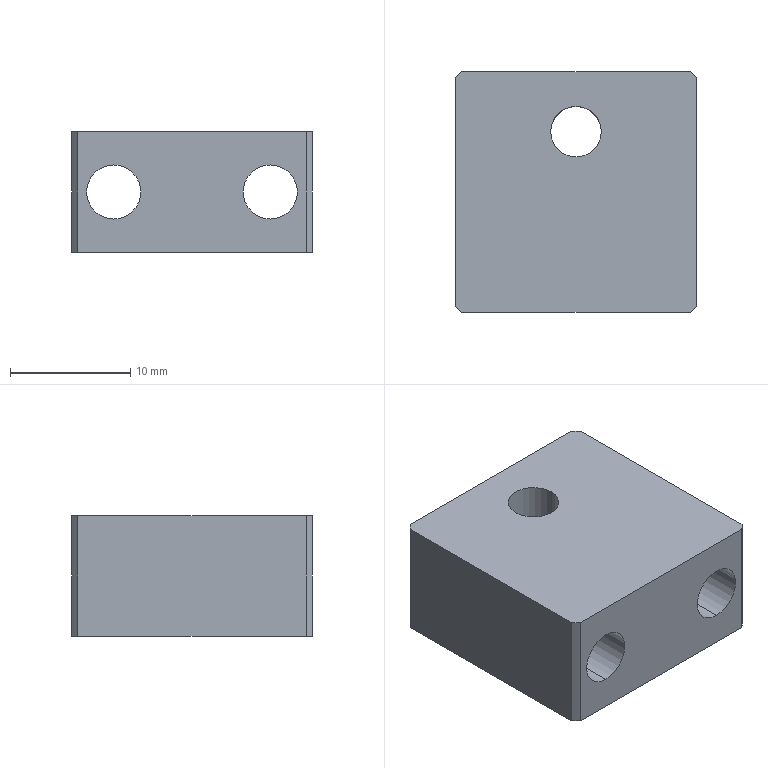Part | SolidWorks | features HoleWzd 2, Chamfer 1, Extrusion 1 | 1 solid | 16 faces | box 20 x 20 x 10 mm | volume 3220 mm3 | plane 10 | cylinder 6 | commonest cylinder face diameters 4.5 x4 4.2 x2
STEP:
#1=CARTESIAN_POINT('',(-6.5,-10.,-2.25));
#2=VERTEX_POINT('',#1);
#3=CARTESIAN_POINT('',(-6.5,-10.,2.25));
#4=VERTEX_POINT('',#3);
#5=CARTESIAN_POINT('',(-6.5,-10.,0.));
#6=DIRECTION('',(0.,1.,0.));
#7=DIRECTION('',(0.,0.,1.));
#8=AXIS2_PLACEMENT_3D('',#5,#6,#7);
#9=CIRCLE('',#8,2.25);
#10=EDGE_CURVE('',#2,#4,#9,.T.);
#11=ORIENTED_EDGE('',*,*,#10,.F.);
#12=CARTESIAN_POINT('',(-6.5,10.,-2.25));
#13=VERTEX_POINT('',#12);
#14=CARTESIAN_POINT('',(-6.5,10.,-2.25));
#15=DIRECTION('',(0.,1.,0.));
#16=VECTOR('',#15,1000.);
#17=LINE('',#14,#16);
#18=EDGE_CURVE('',#2,#13,#17,.T.);
#19=ORIENTED_EDGE('',*,*,#18,.T.);
#20=CARTESIAN_POINT('',(-6.5,10.,2.25));
#21=VERTEX_POINT('',#20);
#22=CARTESIAN_POINT('',(-6.5,10.,0.));
#23=DIRECTION('',(0.,1.,0.));
#24=DIRECTION('',(0.,0.,1.));
#25=AXIS2_PLACEMENT_3D('',#22,#23,#24);
#26=CIRCLE('',#25,2.25);
#27=EDGE_CURVE('',#13,#21,#26,.T.);
#28=ORIENTED_EDGE('',*,*,#27,.T.);
#29=CARTESIAN_POINT('',(-6.5,10.,2.25));
#30=DIRECTION('',(0.,1.,0.));
#31=VECTOR('',#30,1000.);
#32=LINE('',#29,#31);
#33=EDGE_CURVE('',#4,#21,#32,.T.);
#34=ORIENTED_EDGE('',*,*,#33,.F.);
#35=EDGE_LOOP('',(#11,#19,#28,#34));
#36=FACE_OUTER_BOUND('',#35,.T.);
#37=CARTESIAN_POINT('',(-6.5,10.,0.));
#38=DIRECTION('',(0.,1.,0.));
#39=DIRECTION('',(0.,0.,1.));
#40=AXIS2_PLACEMENT_3D('',#37,#38,#39);
#41=CYLINDRICAL_SURFACE('',#40,2.25);
#42=ADVANCED_FACE('',(#36),#41,.F.);
#43=CARTESIAN_POINT('',(6.5,-10.,-2.25));
#44=VERTEX_POINT('',#43);
#45=CARTESIAN_POINT('',(6.5,-10.,2.25));
#46=VERTEX_POINT('',#45);
#47=CARTESIAN_POINT('',(6.5,-10.,0.));
#48=DIRECTION('',(0.,1.,0.));
#49=DIRECTION('',(0.,0.,1.));
#50=AXIS2_PLACEMENT_3D('',#47,#48,#49);
#51=CIRCLE('',#50,2.25);
#52=EDGE_CURVE('',#44,#46,#51,.T.);
#53=ORIENTED_EDGE('',*,*,#52,.F.);
#54=CARTESIAN_POINT('',(6.5,10.,-2.25));
#55=VERTEX_POINT('',#54);
#56=CARTESIAN_POINT('',(6.5,10.,-2.25));
#57=DIRECTION('',(0.,1.,0.));
#58=VECTOR('',#57,1000.);
#59=LINE('',#56,#58);
#60=EDGE_CURVE('',#44,#55,#59,.T.);
#61=ORIENTED_EDGE('',*,*,#60,.T.);
#62=CARTESIAN_POINT('',(6.5,10.,2.25));
#63=VERTEX_POINT('',#62);
#64=CARTESIAN_POINT('',(6.5,10.,0.));
#65=DIRECTION('',(0.,1.,0.));
#66=DIRECTION('',(0.,0.,1.));
#67=AXIS2_PLACEMENT_3D('',#64,#65,#66);
#68=CIRCLE('',#67,2.25);
#69=EDGE_CURVE('',#55,#63,#68,.T.);
#70=ORIENTED_EDGE('',*,*,#69,.T.);
#71=CARTESIAN_POINT('',(6.5,10.,2.25));
#72=DIRECTION('',(0.,1.,0.));
#73=VECTOR('',#72,1000.);
#74=LINE('',#71,#73);
#75=EDGE_CURVE('',#46,#63,#74,.T.);
#76=ORIENTED_EDGE('',*,*,#75,.F.);
#77=EDGE_LOOP('',(#53,#61,#70,#76));
#78=FACE_OUTER_BOUND('',#77,.T.);
#79=CARTESIAN_POINT('',(6.5,10.,0.));
#80=DIRECTION('',(0.,1.,0.));
#81=DIRECTION('',(0.,0.,1.));
#82=AXIS2_PLACEMENT_3D('',#79,#80,#81);
#83=CYLINDRICAL_SURFACE('',#82,2.25);
#84=ADVANCED_FACE('',(#78),#83,.F.);
#85=CARTESIAN_POINT('',(-2.1,5.,-5.));
#86=VERTEX_POINT('',#85);
#87=CARTESIAN_POINT('',(2.1,5.,-5.));
#88=VERTEX_POINT('',#87);
#89=CARTESIAN_POINT('',(0.,5.,-5.));
#90=DIRECTION('',(0.,0.,1.));
#91=DIRECTION('',(1.,0.,0.));
#92=AXIS2_PLACEMENT_3D('',#89,#90,#91);
#93=CIRCLE('',#92,2.1);
#94=EDGE_CURVE('',#86,#88,#93,.T.);
#95=ORIENTED_EDGE('',*,*,#94,.F.);
#96=CARTESIAN_POINT('',(-2.1,5.,5.));
#97=VERTEX_POINT('',#96);
#98=CARTESIAN_POINT('',(-2.1,5.,5.));
#99=DIRECTION('',(0.,0.,1.));
#100=VECTOR('',#99,1000.);
#101=LINE('',#98,#100);
#102=EDGE_CURVE('',#86,#97,#101,.T.);
#103=ORIENTED_EDGE('',*,*,#102,.T.);
#104=CARTESIAN_POINT('',(2.1,5.,5.));
#105=VERTEX_POINT('',#104);
#106=CARTESIAN_POINT('',(0.,5.,5.));
#107=DIRECTION('',(0.,0.,1.));
#108=DIRECTION('',(1.,0.,0.));
#109=AXIS2_PLACEMENT_3D('',#106,#107,#108);
#110=CIRCLE('',#109,2.1);
#111=EDGE_CURVE('',#97,#105,#110,.T.);
#112=ORIENTED_EDGE('',*,*,#111,.T.);
#113=CARTESIAN_POINT('',(2.1,5.,5.));
#114=DIRECTION('',(0.,0.,1.));
#115=VECTOR('',#114,1000.);
#116=LINE('',#113,#115);
#117=EDGE_CURVE('',#88,#105,#116,.T.);
#118=ORIENTED_EDGE('',*,*,#117,.F.);
#119=EDGE_LOOP('',(#95,#103,#112,#118));
#120=FACE_OUTER_BOUND('',#119,.T.);
#121=CARTESIAN_POINT('',(0.,5.,5.));
#122=DIRECTION('',(0.,0.,1.));
#123=DIRECTION('',(1.,0.,0.));
#124=AXIS2_PLACEMENT_3D('',#121,#122,#123);
#125=CYLINDRICAL_SURFACE('',#124,2.1);
#126=ADVANCED_FACE('',(#120),#125,.F.);
#127=CARTESIAN_POINT('',(10.,9.5,5.));
#128=VERTEX_POINT('',#127);
#129=CARTESIAN_POINT('',(10.,-9.5,5.));
#130=VERTEX_POINT('',#129);
#131=CARTESIAN_POINT('',(10.,10.,5.));
#132=DIRECTION('',(0.,-1.,0.));
#133=VECTOR('',#132,1000.);
#134=LINE('',#131,#133);
#135=EDGE_CURVE('',#128,#130,#134,.T.);
#136=ORIENTED_EDGE('',*,*,#135,.T.);
#137=CARTESIAN_POINT('',(10.,-9.5,-5.));
#138=VERTEX_POINT('',#137);
#139=CARTESIAN_POINT('',(10.,-9.5,-5.));
#140=DIRECTION('',(0.,0.,-1.));
#141=VECTOR('',#140,1000.);
#142=LINE('',#139,#141);
#143=EDGE_CURVE('',#130,#138,#142,.T.);
#144=ORIENTED_EDGE('',*,*,#143,.T.);
#145=CARTESIAN_POINT('',(10.,9.5,-5.));
#146=VERTEX_POINT('',#145);
#147=CARTESIAN_POINT('',(10.,10.,-5.));
#148=DIRECTION('',(0.,-1.,0.));
#149=VECTOR('',#148,1000.);
#150=LINE('',#147,#149);
#151=EDGE_CURVE('',#146,#138,#150,.T.);
#152=ORIENTED_EDGE('',*,*,#151,.F.);
#153=CARTESIAN_POINT('',(10.,9.5,5.));
#154=DIRECTION('',(0.,0.,1.));
#155=VECTOR('',#154,1000.);
#156=LINE('',#153,#155);
#157=EDGE_CURVE('',#146,#128,#156,.T.);
#158=ORIENTED_EDGE('',*,*,#157,.T.);
#159=EDGE_LOOP('',(#136,#144,#152,#158));
#160=FACE_OUTER_BOUND('',#159,.T.);
#161=CARTESIAN_POINT('',(10.,10.,5.));
#162=DIRECTION('',(-1.,0.,0.));
#163=DIRECTION('',(0.,0.,1.));
#164=AXIS2_PLACEMENT_3D('',#161,#162,#163);
#165=PLANE('',#164);
#166=ADVANCED_FACE('',(#160),#165,.F.);
#167=CARTESIAN_POINT('',(0.,5.,-5.));
#168=DIRECTION('',(0.,0.,1.));
#169=DIRECTION('',(1.,0.,0.));
#170=AXIS2_PLACEMENT_3D('',#167,#168,#169);
#171=CIRCLE('',#170,2.1);
#172=EDGE_CURVE('',#88,#86,#171,.T.);
#173=ORIENTED_EDGE('',*,*,#172,.T.);
#174=ORIENTED_EDGE('',*,*,#94,.T.);
#175=EDGE_LOOP('',(#173,#174));
#176=FACE_BOUND('',#175,.T.);
#177=ORIENTED_EDGE('',*,*,#151,.T.);
#178=CARTESIAN_POINT('',(9.5,-10.,-5.));
#179=VERTEX_POINT('',#178);
#180=CARTESIAN_POINT('',(10.,-9.5,-5.));
#181=DIRECTION('',(-0.7071,-0.7071,0.));
#182=VECTOR('',#181,1000.);
#183=LINE('',#180,#182);
#184=EDGE_CURVE('',#138,#179,#183,.T.);
#185=ORIENTED_EDGE('',*,*,#184,.T.);
#186=CARTESIAN_POINT('',(-9.5,-10.,-5.));
#187=VERTEX_POINT('',#186);
#188=CARTESIAN_POINT('',(-10.,-10.,-5.));
#189=DIRECTION('',(-1.,0.,0.));
#190=VECTOR('',#189,1000.);
#191=LINE('',#188,#190);
#192=EDGE_CURVE('',#179,#187,#191,.T.);
#193=ORIENTED_EDGE('',*,*,#192,.T.);
#194=CARTESIAN_POINT('',(-10.,-9.5,-5.));
#195=VERTEX_POINT('',#194);
#196=CARTESIAN_POINT('',(-10.,-9.5,-5.));
#197=DIRECTION('',(-0.7071,0.7071,0.));
#198=VECTOR('',#197,1000.);
#199=LINE('',#196,#198);
#200=EDGE_CURVE('',#187,#195,#199,.T.);
#201=ORIENTED_EDGE('',*,*,#200,.T.);
#202=CARTESIAN_POINT('',(-10.,9.5,-5.));
#203=VERTEX_POINT('',#202);
#204=CARTESIAN_POINT('',(-10.,10.,-5.));
#205=DIRECTION('',(0.,-1.,0.));
#206=VECTOR('',#205,1000.);
#207=LINE('',#204,#206);
#208=EDGE_CURVE('',#203,#195,#207,.T.);
#209=ORIENTED_EDGE('',*,*,#208,.F.);
#210=CARTESIAN_POINT('',(-9.5,10.,-5.));
#211=VERTEX_POINT('',#210);
#212=CARTESIAN_POINT('',(-9.5,10.,-5.));
#213=DIRECTION('',(0.7071,0.7071,0.));
#214=VECTOR('',#213,1000.);
#215=LINE('',#212,#214);
#216=EDGE_CURVE('',#203,#211,#215,.T.);
#217=ORIENTED_EDGE('',*,*,#216,.T.);
#218=CARTESIAN_POINT('',(9.5,10.,-5.));
#219=VERTEX_POINT('',#218);
#220=CARTESIAN_POINT('',(-10.,10.,-5.));
#221=DIRECTION('',(-1.,0.,0.));
#222=VECTOR('',#221,1000.);
#223=LINE('',#220,#222);
#224=EDGE_CURVE('',#219,#211,#223,.T.);
#225=ORIENTED_EDGE('',*,*,#224,.F.);
#226=CARTESIAN_POINT('',(9.5,10.,-5.));
#227=DIRECTION('',(0.7071,-0.7071,0.));
#228=VECTOR('',#227,1000.);
#229=LINE('',#226,#228);
#230=EDGE_CURVE('',#219,#146,#229,.T.);
#231=ORIENTED_EDGE('',*,*,#230,.T.);
#232=EDGE_LOOP('',(#177,#185,#193,#201,#209,#217,#225,#231));
#233=FACE_OUTER_BOUND('',#232,.T.);
#234=CARTESIAN_POINT('',(-10.,10.,-5.));
#235=DIRECTION('',(0.,0.,1.));
#236=DIRECTION('',(1.,0.,0.));
#237=AXIS2_PLACEMENT_3D('',#234,#235,#236);
#238=PLANE('',#237);
#239=ADVANCED_FACE('',(#176,#233),#238,.F.);
#240=ORIENTED_EDGE('',*,*,#208,.T.);
#241=CARTESIAN_POINT('',(-10.,-9.5,5.));
#242=VERTEX_POINT('',#241);
#243=CARTESIAN_POINT('',(-10.,-9.5,5.));
#244=DIRECTION('',(0.,0.,1.));
#245=VECTOR('',#244,1000.);
#246=LINE('',#243,#245);
#247=EDGE_CURVE('',#195,#242,#246,.T.);
#248=ORIENTED_EDGE('',*,*,#247,.T.);
#249=CARTESIAN_POINT('',(-10.,9.5,5.));
#250=VERTEX_POINT('',#249);
#251=CARTESIAN_POINT('',(-10.,10.,5.));
#252=DIRECTION('',(0.,-1.,0.));
#253=VECTOR('',#252,1000.);
#254=LINE('',#251,#253);
#255=EDGE_CURVE('',#250,#242,#254,.T.);
#256=ORIENTED_EDGE('',*,*,#255,.F.);
#257=CARTESIAN_POINT('',(-10.,9.5,5.));
#258=DIRECTION('',(0.,0.,-1.));
#259=VECTOR('',#258,1000.);
#260=LINE('',#257,#259);
#261=EDGE_CURVE('',#250,#203,#260,.T.);
#262=ORIENTED_EDGE('',*,*,#261,.T.);
#263=EDGE_LOOP('',(#240,#248,#256,#262));
#264=FACE_OUTER_BOUND('',#263,.T.);
#265=CARTESIAN_POINT('',(-10.,10.,5.));
#266=DIRECTION('',(1.,0.,0.));
#267=DIRECTION('',(0.,0.,-1.));
#268=AXIS2_PLACEMENT_3D('',#265,#266,#267);
#269=PLANE('',#268);
#270=ADVANCED_FACE('',(#264),#269,.F.);
#271=CARTESIAN_POINT('',(0.,5.,5.));
#272=DIRECTION('',(0.,0.,1.));
#273=DIRECTION('',(1.,0.,0.));
#274=AXIS2_PLACEMENT_3D('',#271,#272,#273);
#275=CIRCLE('',#274,2.1);
#276=EDGE_CURVE('',#105,#97,#275,.T.);
#277=ORIENTED_EDGE('',*,*,#276,.F.);
#278=ORIENTED_EDGE('',*,*,#111,.F.);
#279=EDGE_LOOP('',(#277,#278));
#280=FACE_BOUND('',#279,.T.);
#281=CARTESIAN_POINT('',(-9.5,-10.,5.));
#282=VERTEX_POINT('',#281);
#283=CARTESIAN_POINT('',(9.5,-10.,5.));
#284=VERTEX_POINT('',#283);
#285=CARTESIAN_POINT('',(-10.,-10.,5.));
#286=DIRECTION('',(1.,0.,0.));
#287=VECTOR('',#286,1000.);
#288=LINE('',#285,#287);
#289=EDGE_CURVE('',#282,#284,#288,.T.);
#290=ORIENTED_EDGE('',*,*,#289,.T.);
#291=CARTESIAN_POINT('',(10.,-9.5,5.));
#292=DIRECTION('',(0.7071,0.7071,0.));
#293=VECTOR('',#292,1000.);
#294=LINE('',#291,#293);
#295=EDGE_CURVE('',#284,#130,#294,.T.);
#296=ORIENTED_EDGE('',*,*,#295,.T.);
#297=ORIENTED_EDGE('',*,*,#135,.F.);
#298=CARTESIAN_POINT('',(9.5,10.,5.));
#299=VERTEX_POINT('',#298);
#300=CARTESIAN_POINT('',(9.5,10.,5.));
#301=DIRECTION('',(-0.7071,0.7071,0.));
#302=VECTOR('',#301,1000.);
#303=LINE('',#300,#302);
#304=EDGE_CURVE('',#128,#299,#303,.T.);
#305=ORIENTED_EDGE('',*,*,#304,.T.);
#306=CARTESIAN_POINT('',(-9.5,10.,5.));
#307=VERTEX_POINT('',#306);
#308=CARTESIAN_POINT('',(-10.,10.,5.));
#309=DIRECTION('',(1.,0.,0.));
#310=VECTOR('',#309,1000.);
#311=LINE('',#308,#310);
#312=EDGE_CURVE('',#307,#299,#311,.T.);
#313=ORIENTED_EDGE('',*,*,#312,.F.);
#314=CARTESIAN_POINT('',(-9.5,10.,5.));
#315=DIRECTION('',(-0.7071,-0.7071,0.));
#316=VECTOR('',#315,1000.);
#317=LINE('',#314,#316);
#318=EDGE_CURVE('',#307,#250,#317,.T.);
#319=ORIENTED_EDGE('',*,*,#318,.T.);
#320=ORIENTED_EDGE('',*,*,#255,.T.);
#321=CARTESIAN_POINT('',(-10.,-9.5,5.));
#322=DIRECTION('',(0.7071,-0.7071,0.));
#323=VECTOR('',#322,1000.);
#324=LINE('',#321,#323);
#325=EDGE_CURVE('',#242,#282,#324,.T.);
#326=ORIENTED_EDGE('',*,*,#325,.T.);
#327=EDGE_LOOP('',(#290,#296,#297,#305,#313,#319,#320,#326));
#328=FACE_OUTER_BOUND('',#327,.T.);
#329=CARTESIAN_POINT('',(-10.,10.,5.));
#330=DIRECTION('',(0.,0.,-1.));
#331=DIRECTION('',(-1.,0.,0.));
#332=AXIS2_PLACEMENT_3D('',#329,#330,#331);
#333=PLANE('',#332);
#334=ADVANCED_FACE('',(#280,#328),#333,.F.);
#335=CARTESIAN_POINT('',(-6.5,10.,0.));
#336=DIRECTION('',(0.,1.,0.));
#337=DIRECTION('',(0.,0.,1.));
#338=AXIS2_PLACEMENT_3D('',#335,#336,#337);
#339=CIRCLE('',#338,2.25);
#340=EDGE_CURVE('',#21,#13,#339,.T.);
#341=ORIENTED_EDGE('',*,*,#340,.F.);
#342=ORIENTED_EDGE('',*,*,#27,.F.);
#343=EDGE_LOOP('',(#341,#342));
#344=FACE_BOUND('',#343,.T.);
#345=CARTESIAN_POINT('',(6.5,10.,0.));
#346=DIRECTION('',(0.,1.,0.));
#347=DIRECTION('',(0.,0.,1.));
#348=AXIS2_PLACEMENT_3D('',#345,#346,#347);
#349=CIRCLE('',#348,2.25);
#350=EDGE_CURVE('',#63,#55,#349,.T.);
#351=ORIENTED_EDGE('',*,*,#350,.F.);
#352=ORIENTED_EDGE('',*,*,#69,.F.);
#353=EDGE_LOOP('',(#351,#352));
#354=FACE_BOUND('',#353,.T.);
#355=ORIENTED_EDGE('',*,*,#312,.T.);
#356=CARTESIAN_POINT('',(9.5,10.,0.));
#357=DIRECTION('',(0.,0.,-1.));
#358=VECTOR('',#357,1000.);
#359=LINE('',#356,#358);
#360=EDGE_CURVE('',#299,#219,#359,.T.);
#361=ORIENTED_EDGE('',*,*,#360,.T.);
#362=ORIENTED_EDGE('',*,*,#224,.T.);
#363=CARTESIAN_POINT('',(-9.5,10.,0.));
#364=DIRECTION('',(0.,0.,1.));
#365=VECTOR('',#364,1000.);
#366=LINE('',#363,#365);
#367=EDGE_CURVE('',#211,#307,#366,.T.);
#368=ORIENTED_EDGE('',*,*,#367,.T.);
#369=EDGE_LOOP('',(#355,#361,#362,#368));
#370=FACE_OUTER_BOUND('',#369,.T.);
#371=CARTESIAN_POINT('',(0.,10.,0.));
#372=DIRECTION('',(0.,-1.,0.));
#373=DIRECTION('',(0.,0.,-1.));
#374=AXIS2_PLACEMENT_3D('',#371,#372,#373);
#375=PLANE('',#374);
#376=ADVANCED_FACE('',(#344,#354,#370),#375,.F.);
#377=CARTESIAN_POINT('',(-6.5,-10.,0.));
#378=DIRECTION('',(0.,1.,0.));
#379=DIRECTION('',(0.,0.,1.));
#380=AXIS2_PLACEMENT_3D('',#377,#378,#379);
#381=CIRCLE('',#380,2.25);
#382=EDGE_CURVE('',#4,#2,#381,.T.);
#383=ORIENTED_EDGE('',*,*,#382,.T.);
#384=ORIENTED_EDGE('',*,*,#10,.T.);
#385=EDGE_LOOP('',(#383,#384));
#386=FACE_BOUND('',#385,.T.);
#387=CARTESIAN_POINT('',(6.5,-10.,0.));
#388=DIRECTION('',(0.,1.,0.));
#389=DIRECTION('',(0.,0.,1.));
#390=AXIS2_PLACEMENT_3D('',#387,#388,#389);
#391=CIRCLE('',#390,2.25);
#392=EDGE_CURVE('',#46,#44,#391,.T.);
#393=ORIENTED_EDGE('',*,*,#392,.T.);
#394=ORIENTED_EDGE('',*,*,#52,.T.);
#395=EDGE_LOOP('',(#393,#394));
#396=FACE_BOUND('',#395,.T.);
#397=ORIENTED_EDGE('',*,*,#192,.F.);
#398=CARTESIAN_POINT('',(9.5,-10.,5.));
#399=DIRECTION('',(0.,0.,1.));
#400=VECTOR('',#399,1000.);
#401=LINE('',#398,#400);
#402=EDGE_CURVE('',#179,#284,#401,.T.);
#403=ORIENTED_EDGE('',*,*,#402,.T.);
#404=ORIENTED_EDGE('',*,*,#289,.F.);
#405=CARTESIAN_POINT('',(-9.5,-10.,-5.));
#406=DIRECTION('',(0.,0.,-1.));
#407=VECTOR('',#406,1000.);
#408=LINE('',#405,#407);
#409=EDGE_CURVE('',#282,#187,#408,.T.);
#410=ORIENTED_EDGE('',*,*,#409,.T.);
#411=EDGE_LOOP('',(#397,#403,#404,#410));
#412=FACE_OUTER_BOUND('',#411,.T.);
#413=CARTESIAN_POINT('',(0.,-10.,0.));
#414=DIRECTION('',(0.,-1.,0.));
#415=DIRECTION('',(0.,0.,-1.));
#416=AXIS2_PLACEMENT_3D('',#413,#414,#415);
#417=PLANE('',#416);
#418=ADVANCED_FACE('',(#386,#396,#412),#417,.T.);
#419=ORIENTED_EDGE('',*,*,#102,.F.);
#420=ORIENTED_EDGE('',*,*,#172,.F.);
#421=ORIENTED_EDGE('',*,*,#117,.T.);
#422=ORIENTED_EDGE('',*,*,#276,.T.);
#423=EDGE_LOOP('',(#419,#420,#421,#422));
#424=FACE_OUTER_BOUND('',#423,.T.);
#425=CARTESIAN_POINT('',(0.,5.,5.));
#426=DIRECTION('',(0.,0.,1.));
#427=DIRECTION('',(1.,0.,0.));
#428=AXIS2_PLACEMENT_3D('',#425,#426,#427);
#429=CYLINDRICAL_SURFACE('',#428,2.1);
#430=ADVANCED_FACE('',(#424),#429,.F.);
#431=ORIENTED_EDGE('',*,*,#60,.F.);
#432=ORIENTED_EDGE('',*,*,#392,.F.);
#433=ORIENTED_EDGE('',*,*,#75,.T.);
#434=ORIENTED_EDGE('',*,*,#350,.T.);
#435=EDGE_LOOP('',(#431,#432,#433,#434));
#436=FACE_OUTER_BOUND('',#435,.T.);
#437=CARTESIAN_POINT('',(6.5,10.,0.));
#438=DIRECTION('',(0.,1.,0.));
#439=DIRECTION('',(0.,0.,1.));
#440=AXIS2_PLACEMENT_3D('',#437,#438,#439);
#441=CYLINDRICAL_SURFACE('',#440,2.25);
#442=ADVANCED_FACE('',(#436),#441,.F.);
#443=ORIENTED_EDGE('',*,*,#18,.F.);
#444=ORIENTED_EDGE('',*,*,#382,.F.);
#445=ORIENTED_EDGE('',*,*,#33,.T.);
#446=ORIENTED_EDGE('',*,*,#340,.T.);
#447=EDGE_LOOP('',(#443,#444,#445,#446));
#448=FACE_OUTER_BOUND('',#447,.T.);
#449=CARTESIAN_POINT('',(-6.5,10.,0.));
#450=DIRECTION('',(0.,1.,0.));
#451=DIRECTION('',(0.,0.,1.));
#452=AXIS2_PLACEMENT_3D('',#449,#450,#451);
#453=CYLINDRICAL_SURFACE('',#452,2.25);
#454=ADVANCED_FACE('',(#448),#453,.F.);
#455=ORIENTED_EDGE('',*,*,#295,.F.);
#456=ORIENTED_EDGE('',*,*,#402,.F.);
#457=ORIENTED_EDGE('',*,*,#184,.F.);
#458=ORIENTED_EDGE('',*,*,#143,.F.);
#459=EDGE_LOOP('',(#455,#456,#457,#458));
#460=FACE_OUTER_BOUND('',#459,.T.);
#461=CARTESIAN_POINT('',(10.,-9.5,5.));
#462=DIRECTION('',(0.7071,-0.7071,0.));
#463=DIRECTION('',(0.,0.,1.));
#464=AXIS2_PLACEMENT_3D('',#461,#462,#463);
#465=PLANE('',#464);
#466=ADVANCED_FACE('',(#460),#465,.T.);
#467=ORIENTED_EDGE('',*,*,#200,.F.);
#468=ORIENTED_EDGE('',*,*,#409,.F.);
#469=ORIENTED_EDGE('',*,*,#325,.F.);
#470=ORIENTED_EDGE('',*,*,#247,.F.);
#471=EDGE_LOOP('',(#467,#468,#469,#470));
#472=FACE_OUTER_BOUND('',#471,.T.);
#473=CARTESIAN_POINT('',(-10.,-9.5,5.));
#474=DIRECTION('',(-0.7071,-0.7071,0.));
#475=DIRECTION('',(0.,0.,-1.));
#476=AXIS2_PLACEMENT_3D('',#473,#474,#475);
#477=PLANE('',#476);
#478=ADVANCED_FACE('',(#472),#477,.T.);
#479=ORIENTED_EDGE('',*,*,#304,.F.);
#480=ORIENTED_EDGE('',*,*,#157,.F.);
#481=ORIENTED_EDGE('',*,*,#230,.F.);
#482=ORIENTED_EDGE('',*,*,#360,.F.);
#483=EDGE_LOOP('',(#479,#480,#481,#482));
#484=FACE_OUTER_BOUND('',#483,.T.);
#485=CARTESIAN_POINT('',(9.5,10.,0.));
#486=DIRECTION('',(-0.7071,-0.7071,0.));
#487=DIRECTION('',(0.,0.,-1.));
#488=AXIS2_PLACEMENT_3D('',#485,#486,#487);
#489=PLANE('',#488);
#490=ADVANCED_FACE('',(#484),#489,.F.);
#491=ORIENTED_EDGE('',*,*,#216,.F.);
#492=ORIENTED_EDGE('',*,*,#261,.F.);
#493=ORIENTED_EDGE('',*,*,#318,.F.);
#494=ORIENTED_EDGE('',*,*,#367,.F.);
#495=EDGE_LOOP('',(#491,#492,#493,#494));
#496=FACE_OUTER_BOUND('',#495,.T.);
#497=CARTESIAN_POINT('',(-9.5,10.,0.));
#498=DIRECTION('',(0.7071,-0.7071,0.));
#499=DIRECTION('',(0.,0.,1.));
#500=AXIS2_PLACEMENT_3D('',#497,#498,#499);
#501=PLANE('',#500);
#502=ADVANCED_FACE('',(#496),#501,.F.);
#503=CLOSED_SHELL('',(#42,#84,#126,#166,#239,#270,#334,#376,#418,#430,#442,#454,#466,#478,#490,#502));
#504=MANIFOLD_SOLID_BREP('',#503);
#505=CARTESIAN_POINT('',(0.,0.,0.));
#506=DIRECTION('',(0.,0.,1.));
#507=DIRECTION('',(1.,0.,0.));
#508=AXIS2_PLACEMENT_3D('',#505,#506,#507);
#509=(LENGTH_UNIT()NAMED_UNIT(*)SI_UNIT(.MILLI.,.METRE.));
#510=UNCERTAINTY_MEASURE_WITH_UNIT(LENGTH_MEASURE(0.00001),#509,'','');
#511=(NAMED_UNIT(*)PLANE_ANGLE_UNIT()SI_UNIT($,.RADIAN.));
#512=(NAMED_UNIT(*)SI_UNIT($,.STERADIAN.)SOLID_ANGLE_UNIT());
#513=(GEOMETRIC_REPRESENTATION_CONTEXT(3)GLOBAL_UNCERTAINTY_ASSIGNED_CONTEXT((#510))GLOBAL_UNIT_ASSIGNED_CONTEXT((#509,#511,#512))REPRESENTATION_CONTEXT('',''));
#514=ADVANCED_BREP_SHAPE_REPRESENTATION('',(#504,#508),#513);